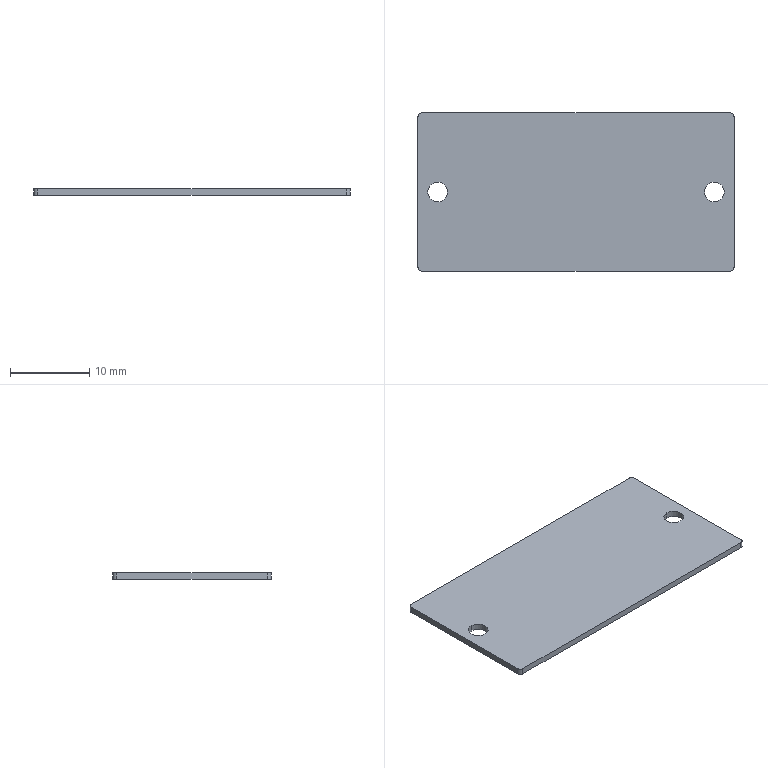Part | STEP file | Nameplate | 1 solid | 14 faces | box 40 x 20 x 0.8 mm | volume 631.974 mm3 | cylinder 8 | plane 6 | commonest cylinder face diameters 1 x4 2.5 x4
STEP:
#1=CARTESIAN_POINT('',(0.,0.,0.));
#2=DIRECTION('',(0.,0.,1.));
#3=DIRECTION('',(1.,0.,0.));
#4=AXIS2_PLACEMENT_3D('',#1,#2,#3);
#5=CARTESIAN_POINT('',(37.5,11.25,0.8));
#6=VERTEX_POINT('',#5);
#7=CARTESIAN_POINT('',(37.5,11.25,0.));
#8=VERTEX_POINT('',#7);
#9=CARTESIAN_POINT('',(37.5,11.25,0.8));
#10=DIRECTION('',(0.,0.,-1.));
#11=VECTOR('',#10,1.);
#12=LINE('',#9,#11);
#13=CARTESIAN_POINT('',(37.5,10.,0.8));
#14=DIRECTION('',(0.,0.,-1.));
#15=DIRECTION('',(0.,1.,0.));
#16=AXIS2_PLACEMENT_3D('',#13,#14,#15);
#17=CYLINDRICAL_SURFACE('',#16,1.25);
#18=CARTESIAN_POINT('',(6.283,0.));
#19=DIRECTION('',(0.,1.));
#20=VECTOR('',#19,1.);
#21=LINE('',#18,#20);
#22=(GEOMETRIC_REPRESENTATION_CONTEXT(2)PARAMETRIC_REPRESENTATION_CONTEXT()REPRESENTATION_CONTEXT('',''));
#23=DEFINITIONAL_REPRESENTATION('',(#21),#22);
#24=PCURVE('',#17,#23);
#25=CARTESIAN_POINT('',(37.5,10.,0.8));
#26=DIRECTION('',(0.,0.,-1.));
#27=DIRECTION('',(0.,1.,0.));
#28=AXIS2_PLACEMENT_3D('',#25,#26,#27);
#29=CYLINDRICAL_SURFACE('',#28,1.25);
#30=CARTESIAN_POINT('',(0.,0.));
#31=DIRECTION('',(0.,1.));
#32=VECTOR('',#31,1.);
#33=LINE('',#30,#32);
#34=(GEOMETRIC_REPRESENTATION_CONTEXT(2)PARAMETRIC_REPRESENTATION_CONTEXT()REPRESENTATION_CONTEXT('',''));
#35=DEFINITIONAL_REPRESENTATION('',(#33),#34);
#36=PCURVE('',#29,#35);
#37=SURFACE_CURVE('',#12,(#24,#36),.PCURVE_S1.);
#38=EDGE_CURVE('',#6,#8,#37,.T.);
#39=ORIENTED_EDGE('',*,*,#38,.T.);
#40=CARTESIAN_POINT('',(37.5,8.75,0.));
#41=VERTEX_POINT('',#40);
#42=CARTESIAN_POINT('',(37.5,10.,0.));
#43=DIRECTION('',(0.,0.,1.));
#44=DIRECTION('',(0.,-1.,0.));
#45=AXIS2_PLACEMENT_3D('',#42,#43,#44);
#46=CIRCLE('',#45,1.25);
#47=CARTESIAN_POINT('',(9.425,0.8));
#48=DIRECTION('',(-1.,0.));
#49=VECTOR('',#48,1.);
#50=LINE('',#47,#49);
#51=(GEOMETRIC_REPRESENTATION_CONTEXT(2)PARAMETRIC_REPRESENTATION_CONTEXT()REPRESENTATION_CONTEXT('',''));
#52=DEFINITIONAL_REPRESENTATION('',(#50),#51);
#53=PCURVE('',#17,#52);
#54=CARTESIAN_POINT('',(20.,0.,0.));
#55=DIRECTION('',(0.,0.,-1.));
#56=DIRECTION('',(0.,1.,0.));
#57=AXIS2_PLACEMENT_3D('',#54,#55,#56);
#58=PLANE('',#57);
#59=CARTESIAN_POINT('',(8.75,17.5));
#60=CARTESIAN_POINT('',(8.75,19.665));
#61=CARTESIAN_POINT('',(10.625,18.583));
#62=CARTESIAN_POINT('',(12.5,17.5));
#63=CARTESIAN_POINT('',(10.625,16.417));
#64=CARTESIAN_POINT('',(8.75,15.335));
#65=CARTESIAN_POINT('',(8.75,17.5));
#66=(BOUNDED_CURVE()B_SPLINE_CURVE(2,(#59,#60,#61,#62,#63,#64,#65),.UNSPECIFIED.,.T.,.F.)B_SPLINE_CURVE_WITH_KNOTS((1,2,2,2,2,1),(-2.094,0.,2.094,4.189,6.283,8.378),.UNSPECIFIED.)CURVE()GEOMETRIC_REPRESENTATION_ITEM()RATIONAL_B_SPLINE_CURVE((1.,0.5,1.,0.5,1.,0.5,1.))REPRESENTATION_ITEM(''));
#67=(GEOMETRIC_REPRESENTATION_CONTEXT(2)PARAMETRIC_REPRESENTATION_CONTEXT()REPRESENTATION_CONTEXT('',''));
#68=DEFINITIONAL_REPRESENTATION('',(#66),#67);
#69=PCURVE('',#58,#68);
#70=SURFACE_CURVE('',#46,(#53,#69),.PCURVE_S1.);
#71=EDGE_CURVE('',#8,#41,#70,.T.);
#72=ORIENTED_EDGE('',*,*,#71,.T.);
#73=CARTESIAN_POINT('',(37.5,8.75,0.8));
#74=VERTEX_POINT('',#73);
#75=CARTESIAN_POINT('',(37.5,8.75,0.8));
#76=DIRECTION('',(0.,0.,-1.));
#77=VECTOR('',#76,1.);
#78=LINE('',#75,#77);
#79=CARTESIAN_POINT('',(3.142,0.));
#80=DIRECTION('',(0.,1.));
#81=VECTOR('',#80,1.);
#82=LINE('',#79,#81);
#83=(GEOMETRIC_REPRESENTATION_CONTEXT(2)PARAMETRIC_REPRESENTATION_CONTEXT()REPRESENTATION_CONTEXT('',''));
#84=DEFINITIONAL_REPRESENTATION('',(#82),#83);
#85=PCURVE('',#17,#84);
#86=CARTESIAN_POINT('',(3.142,0.));
#87=DIRECTION('',(0.,1.));
#88=VECTOR('',#87,1.);
#89=LINE('',#86,#88);
#90=(GEOMETRIC_REPRESENTATION_CONTEXT(2)PARAMETRIC_REPRESENTATION_CONTEXT()REPRESENTATION_CONTEXT('',''));
#91=DEFINITIONAL_REPRESENTATION('',(#89),#90);
#92=PCURVE('',#29,#91);
#93=SURFACE_CURVE('',#78,(#85,#92),.PCURVE_S1.);
#94=EDGE_CURVE('',#74,#41,#93,.T.);
#95=ORIENTED_EDGE('',*,*,#94,.F.);
#96=CARTESIAN_POINT('',(37.5,10.,0.8));
#97=DIRECTION('',(0.,0.,-1.));
#98=DIRECTION('',(0.,1.,0.));
#99=AXIS2_PLACEMENT_3D('',#96,#97,#98);
#100=CIRCLE('',#99,1.25);
#101=CARTESIAN_POINT('',(0.,0.));
#102=DIRECTION('',(1.,0.));
#103=VECTOR('',#102,1.);
#104=LINE('',#101,#103);
#105=(GEOMETRIC_REPRESENTATION_CONTEXT(2)PARAMETRIC_REPRESENTATION_CONTEXT()REPRESENTATION_CONTEXT('',''));
#106=DEFINITIONAL_REPRESENTATION('',(#104),#105);
#107=PCURVE('',#17,#106);
#108=CARTESIAN_POINT('',(20.,0.,0.8));
#109=DIRECTION('',(0.,0.,1.));
#110=DIRECTION('',(0.,-1.,0.));
#111=AXIS2_PLACEMENT_3D('',#108,#109,#110);
#112=PLANE('',#111);
#113=CARTESIAN_POINT('',(-11.25,17.5));
#114=CARTESIAN_POINT('',(-11.25,19.665));
#115=CARTESIAN_POINT('',(-9.375,18.583));
#116=CARTESIAN_POINT('',(-7.5,17.5));
#117=CARTESIAN_POINT('',(-9.375,16.417));
#118=CARTESIAN_POINT('',(-11.25,15.335));
#119=CARTESIAN_POINT('',(-11.25,17.5));
#120=(BOUNDED_CURVE()B_SPLINE_CURVE(2,(#113,#114,#115,#116,#117,#118,#119),.UNSPECIFIED.,.T.,.F.)B_SPLINE_CURVE_WITH_KNOTS((1,2,2,2,2,1),(-2.094,0.,2.094,4.189,6.283,8.378),.UNSPECIFIED.)CURVE()GEOMETRIC_REPRESENTATION_ITEM()RATIONAL_B_SPLINE_CURVE((1.,0.5,1.,0.5,1.,0.5,1.))REPRESENTATION_ITEM(''));
#121=(GEOMETRIC_REPRESENTATION_CONTEXT(2)PARAMETRIC_REPRESENTATION_CONTEXT()REPRESENTATION_CONTEXT('',''));
#122=DEFINITIONAL_REPRESENTATION('',(#120),#121);
#123=PCURVE('',#112,#122);
#124=SURFACE_CURVE('',#100,(#107,#123),.PCURVE_S1.);
#125=EDGE_CURVE('',#74,#6,#124,.T.);
#126=ORIENTED_EDGE('',*,*,#125,.T.);
#127=EDGE_LOOP('',(#39,#72,#95,#126));
#128=FACE_BOUND('',#127,.F.);
#129=ADVANCED_FACE('',(#128),#17,.F.);
#130=CARTESIAN_POINT('',(2.5,11.25,0.8));
#131=VERTEX_POINT('',#130);
#132=CARTESIAN_POINT('',(2.5,11.25,0.));
#133=VERTEX_POINT('',#132);
#134=CARTESIAN_POINT('',(2.5,11.25,0.8));
#135=DIRECTION('',(0.,0.,-1.));
#136=VECTOR('',#135,1.);
#137=LINE('',#134,#136);
#138=CARTESIAN_POINT('',(2.5,10.,0.8));
#139=DIRECTION('',(0.,0.,-1.));
#140=DIRECTION('',(0.,1.,0.));
#141=AXIS2_PLACEMENT_3D('',#138,#139,#140);
#142=CYLINDRICAL_SURFACE('',#141,1.25);
#143=CARTESIAN_POINT('',(6.283,0.));
#144=DIRECTION('',(0.,1.));
#145=VECTOR('',#144,1.);
#146=LINE('',#143,#145);
#147=(GEOMETRIC_REPRESENTATION_CONTEXT(2)PARAMETRIC_REPRESENTATION_CONTEXT()REPRESENTATION_CONTEXT('',''));
#148=DEFINITIONAL_REPRESENTATION('',(#146),#147);
#149=PCURVE('',#142,#148);
#150=CARTESIAN_POINT('',(2.5,10.,0.8));
#151=DIRECTION('',(0.,0.,-1.));
#152=DIRECTION('',(0.,1.,0.));
#153=AXIS2_PLACEMENT_3D('',#150,#151,#152);
#154=CYLINDRICAL_SURFACE('',#153,1.25);
#155=CARTESIAN_POINT('',(0.,0.));
#156=DIRECTION('',(0.,1.));
#157=VECTOR('',#156,1.);
#158=LINE('',#155,#157);
#159=(GEOMETRIC_REPRESENTATION_CONTEXT(2)PARAMETRIC_REPRESENTATION_CONTEXT()REPRESENTATION_CONTEXT('',''));
#160=DEFINITIONAL_REPRESENTATION('',(#158),#159);
#161=PCURVE('',#154,#160);
#162=SURFACE_CURVE('',#137,(#149,#161),.PCURVE_S1.);
#163=EDGE_CURVE('',#131,#133,#162,.T.);
#164=ORIENTED_EDGE('',*,*,#163,.T.);
#165=CARTESIAN_POINT('',(2.5,8.75,0.));
#166=VERTEX_POINT('',#165);
#167=CARTESIAN_POINT('',(2.5,10.,0.));
#168=DIRECTION('',(0.,0.,1.));
#169=DIRECTION('',(0.,-1.,0.));
#170=AXIS2_PLACEMENT_3D('',#167,#168,#169);
#171=CIRCLE('',#170,1.25);
#172=CARTESIAN_POINT('',(9.425,0.8));
#173=DIRECTION('',(-1.,0.));
#174=VECTOR('',#173,1.);
#175=LINE('',#172,#174);
#176=(GEOMETRIC_REPRESENTATION_CONTEXT(2)PARAMETRIC_REPRESENTATION_CONTEXT()REPRESENTATION_CONTEXT('',''));
#177=DEFINITIONAL_REPRESENTATION('',(#175),#176);
#178=PCURVE('',#142,#177);
#179=CARTESIAN_POINT('',(8.75,-17.5));
#180=CARTESIAN_POINT('',(8.75,-15.335));
#181=CARTESIAN_POINT('',(10.625,-16.417));
#182=CARTESIAN_POINT('',(12.5,-17.5));
#183=CARTESIAN_POINT('',(10.625,-18.583));
#184=CARTESIAN_POINT('',(8.75,-19.665));
#185=CARTESIAN_POINT('',(8.75,-17.5));
#186=(BOUNDED_CURVE()B_SPLINE_CURVE(2,(#179,#180,#181,#182,#183,#184,#185),.UNSPECIFIED.,.T.,.F.)B_SPLINE_CURVE_WITH_KNOTS((1,2,2,2,2,1),(-2.094,0.,2.094,4.189,6.283,8.378),.UNSPECIFIED.)CURVE()GEOMETRIC_REPRESENTATION_ITEM()RATIONAL_B_SPLINE_CURVE((1.,0.5,1.,0.5,1.,0.5,1.))REPRESENTATION_ITEM(''));
#187=(GEOMETRIC_REPRESENTATION_CONTEXT(2)PARAMETRIC_REPRESENTATION_CONTEXT()REPRESENTATION_CONTEXT('',''));
#188=DEFINITIONAL_REPRESENTATION('',(#186),#187);
#189=PCURVE('',#58,#188);
#190=SURFACE_CURVE('',#171,(#178,#189),.PCURVE_S1.);
#191=EDGE_CURVE('',#133,#166,#190,.T.);
#192=ORIENTED_EDGE('',*,*,#191,.T.);
#193=CARTESIAN_POINT('',(2.5,8.75,0.8));
#194=VERTEX_POINT('',#193);
#195=CARTESIAN_POINT('',(2.5,8.75,0.8));
#196=DIRECTION('',(0.,0.,-1.));
#197=VECTOR('',#196,1.);
#198=LINE('',#195,#197);
#199=CARTESIAN_POINT('',(3.142,0.));
#200=DIRECTION('',(0.,1.));
#201=VECTOR('',#200,1.);
#202=LINE('',#199,#201);
#203=(GEOMETRIC_REPRESENTATION_CONTEXT(2)PARAMETRIC_REPRESENTATION_CONTEXT()REPRESENTATION_CONTEXT('',''));
#204=DEFINITIONAL_REPRESENTATION('',(#202),#203);
#205=PCURVE('',#142,#204);
#206=CARTESIAN_POINT('',(3.142,0.));
#207=DIRECTION('',(0.,1.));
#208=VECTOR('',#207,1.);
#209=LINE('',#206,#208);
#210=(GEOMETRIC_REPRESENTATION_CONTEXT(2)PARAMETRIC_REPRESENTATION_CONTEXT()REPRESENTATION_CONTEXT('',''));
#211=DEFINITIONAL_REPRESENTATION('',(#209),#210);
#212=PCURVE('',#154,#211);
#213=SURFACE_CURVE('',#198,(#205,#212),.PCURVE_S1.);
#214=EDGE_CURVE('',#194,#166,#213,.T.);
#215=ORIENTED_EDGE('',*,*,#214,.F.);
#216=CARTESIAN_POINT('',(2.5,10.,0.8));
#217=DIRECTION('',(0.,0.,-1.));
#218=DIRECTION('',(0.,1.,0.));
#219=AXIS2_PLACEMENT_3D('',#216,#217,#218);
#220=CIRCLE('',#219,1.25);
#221=CARTESIAN_POINT('',(0.,0.));
#222=DIRECTION('',(1.,0.));
#223=VECTOR('',#222,1.);
#224=LINE('',#221,#223);
#225=(GEOMETRIC_REPRESENTATION_CONTEXT(2)PARAMETRIC_REPRESENTATION_CONTEXT()REPRESENTATION_CONTEXT('',''));
#226=DEFINITIONAL_REPRESENTATION('',(#224),#225);
#227=PCURVE('',#142,#226);
#228=CARTESIAN_POINT('',(-11.25,-17.5));
#229=CARTESIAN_POINT('',(-11.25,-15.335));
#230=CARTESIAN_POINT('',(-9.375,-16.417));
#231=CARTESIAN_POINT('',(-7.5,-17.5));
#232=CARTESIAN_POINT('',(-9.375,-18.583));
#233=CARTESIAN_POINT('',(-11.25,-19.665));
#234=CARTESIAN_POINT('',(-11.25,-17.5));
#235=(BOUNDED_CURVE()B_SPLINE_CURVE(2,(#228,#229,#230,#231,#232,#233,#234),.UNSPECIFIED.,.T.,.F.)B_SPLINE_CURVE_WITH_KNOTS((1,2,2,2,2,1),(-2.094,0.,2.094,4.189,6.283,8.378),.UNSPECIFIED.)CURVE()GEOMETRIC_REPRESENTATION_ITEM()RATIONAL_B_SPLINE_CURVE((1.,0.5,1.,0.5,1.,0.5,1.))REPRESENTATION_ITEM(''));
#236=(GEOMETRIC_REPRESENTATION_CONTEXT(2)PARAMETRIC_REPRESENTATION_CONTEXT()REPRESENTATION_CONTEXT('',''));
#237=DEFINITIONAL_REPRESENTATION('',(#235),#236);
#238=PCURVE('',#112,#237);
#239=SURFACE_CURVE('',#220,(#227,#238),.PCURVE_S1.);
#240=EDGE_CURVE('',#194,#131,#239,.T.);
#241=ORIENTED_EDGE('',*,*,#240,.T.);
#242=EDGE_LOOP('',(#164,#192,#215,#241));
#243=FACE_BOUND('',#242,.F.);
#244=ADVANCED_FACE('',(#243),#142,.F.);
#245=CARTESIAN_POINT('',(0.5,20.,0.));
#246=VERTEX_POINT('',#245);
#247=CARTESIAN_POINT('',(39.5,20.,0.));
#248=VERTEX_POINT('',#247);
#249=CARTESIAN_POINT('',(20.,20.,0.));
#250=DIRECTION('',(1.,0.,0.));
#251=VECTOR('',#250,1.);
#252=LINE('',#249,#251);
#253=CARTESIAN_POINT('',(20.,20.,0.4));
#254=DIRECTION('',(0.,1.,0.));
#255=DIRECTION('',(1.,0.,0.));
#256=AXIS2_PLACEMENT_3D('',#253,#254,#255);
#257=PLANE('',#256);
#258=CARTESIAN_POINT('',(0.,0.4));
#259=DIRECTION('',(1.,0.));
#260=VECTOR('',#259,1.);
#261=LINE('',#258,#260);
#262=(GEOMETRIC_REPRESENTATION_CONTEXT(2)PARAMETRIC_REPRESENTATION_CONTEXT()REPRESENTATION_CONTEXT('',''));
#263=DEFINITIONAL_REPRESENTATION('',(#261),#262);
#264=PCURVE('',#257,#263);
#265=CARTESIAN_POINT('',(20.,0.));
#266=DIRECTION('',(0.,1.));
#267=VECTOR('',#266,1.);
#268=LINE('',#265,#267);
#269=(GEOMETRIC_REPRESENTATION_CONTEXT(2)PARAMETRIC_REPRESENTATION_CONTEXT()REPRESENTATION_CONTEXT('',''));
#270=DEFINITIONAL_REPRESENTATION('',(#268),#269);
#271=PCURVE('',#58,#270);
#272=SURFACE_CURVE('',#252,(#264,#271),.PCURVE_S1.);
#273=EDGE_CURVE('',#246,#248,#272,.T.);
#274=ORIENTED_EDGE('',*,*,#273,.F.);
#275=CARTESIAN_POINT('',(0.5,20.,0.8));
#276=VERTEX_POINT('',#275);
#277=CARTESIAN_POINT('',(0.5,20.,0.4));
#278=DIRECTION('',(0.,0.,1.));
#279=VECTOR('',#278,1.);
#280=LINE('',#277,#279);
#281=CARTESIAN_POINT('',(-19.5,0.));
#282=DIRECTION('',(0.,-1.));
#283=VECTOR('',#282,1.);
#284=LINE('',#281,#283);
#285=(GEOMETRIC_REPRESENTATION_CONTEXT(2)PARAMETRIC_REPRESENTATION_CONTEXT()REPRESENTATION_CONTEXT('',''));
#286=DEFINITIONAL_REPRESENTATION('',(#284),#285);
#287=PCURVE('',#257,#286);
#288=CARTESIAN_POINT('',(0.5,19.5,0.4));
#289=DIRECTION('',(0.,0.,-1.));
#290=DIRECTION('',(0.,1.,0.));
#291=AXIS2_PLACEMENT_3D('',#288,#289,#290);
#292=CYLINDRICAL_SURFACE('',#291,0.5);
#293=CARTESIAN_POINT('',(6.283,0.));
#294=DIRECTION('',(0.,-1.));
#295=VECTOR('',#294,1.);
#296=LINE('',#293,#295);
#297=(GEOMETRIC_REPRESENTATION_CONTEXT(2)PARAMETRIC_REPRESENTATION_CONTEXT()REPRESENTATION_CONTEXT('',''));
#298=DEFINITIONAL_REPRESENTATION('',(#296),#297);
#299=PCURVE('',#292,#298);
#300=SURFACE_CURVE('',#280,(#287,#299),.PCURVE_S1.);
#301=EDGE_CURVE('',#246,#276,#300,.T.);
#302=ORIENTED_EDGE('',*,*,#301,.T.);
#303=CARTESIAN_POINT('',(39.5,20.,0.8));
#304=VERTEX_POINT('',#303);
#305=CARTESIAN_POINT('',(20.,20.,0.8));
#306=DIRECTION('',(-1.,0.,0.));
#307=VECTOR('',#306,1.);
#308=LINE('',#305,#307);
#309=CARTESIAN_POINT('',(0.,-0.4));
#310=DIRECTION('',(-1.,0.));
#311=VECTOR('',#310,1.);
#312=LINE('',#309,#311);
#313=(GEOMETRIC_REPRESENTATION_CONTEXT(2)PARAMETRIC_REPRESENTATION_CONTEXT()REPRESENTATION_CONTEXT('',''));
#314=DEFINITIONAL_REPRESENTATION('',(#312),#313);
#315=PCURVE('',#257,#314);
#316=CARTESIAN_POINT('',(-20.,0.));
#317=DIRECTION('',(0.,-1.));
#318=VECTOR('',#317,1.);
#319=LINE('',#316,#318);
#320=(GEOMETRIC_REPRESENTATION_CONTEXT(2)PARAMETRIC_REPRESENTATION_CONTEXT()REPRESENTATION_CONTEXT('',''));
#321=DEFINITIONAL_REPRESENTATION('',(#319),#320);
#322=PCURVE('',#112,#321);
#323=SURFACE_CURVE('',#308,(#315,#322),.PCURVE_S1.);
#324=EDGE_CURVE('',#304,#276,#323,.T.);
#325=ORIENTED_EDGE('',*,*,#324,.F.);
#326=CARTESIAN_POINT('',(39.5,20.,0.4));
#327=DIRECTION('',(0.,0.,-1.));
#328=VECTOR('',#327,1.);
#329=LINE('',#326,#328);
#330=CARTESIAN_POINT('',(19.5,0.));
#331=DIRECTION('',(0.,1.));
#332=VECTOR('',#331,1.);
#333=LINE('',#330,#332);
#334=(GEOMETRIC_REPRESENTATION_CONTEXT(2)PARAMETRIC_REPRESENTATION_CONTEXT()REPRESENTATION_CONTEXT('',''));
#335=DEFINITIONAL_REPRESENTATION('',(#333),#334);
#336=PCURVE('',#257,#335);
#337=CARTESIAN_POINT('',(39.5,19.5,0.4));
#338=DIRECTION('',(0.,0.,1.));
#339=DIRECTION('',(0.,-1.,0.));
#340=AXIS2_PLACEMENT_3D('',#337,#338,#339);
#341=CYLINDRICAL_SURFACE('',#340,0.5);
#342=CARTESIAN_POINT('',(3.142,0.));
#343=DIRECTION('',(0.,-1.));
#344=VECTOR('',#343,1.);
#345=LINE('',#342,#344);
#346=(GEOMETRIC_REPRESENTATION_CONTEXT(2)PARAMETRIC_REPRESENTATION_CONTEXT()REPRESENTATION_CONTEXT('',''));
#347=DEFINITIONAL_REPRESENTATION('',(#345),#346);
#348=PCURVE('',#341,#347);
#349=SURFACE_CURVE('',#329,(#336,#348),.PCURVE_S1.);
#350=EDGE_CURVE('',#304,#248,#349,.T.);
#351=ORIENTED_EDGE('',*,*,#350,.T.);
#352=EDGE_LOOP('',(#274,#302,#325,#351));
#353=FACE_BOUND('',#352,.T.);
#354=ADVANCED_FACE('',(#353),#257,.T.);
#355=CARTESIAN_POINT('',(37.5,10.,0.8));
#356=DIRECTION('',(0.,0.,-1.));
#357=DIRECTION('',(0.,1.,0.));
#358=AXIS2_PLACEMENT_3D('',#355,#356,#357);
#359=CIRCLE('',#358,1.25);
#360=CARTESIAN_POINT('',(-11.25,17.5));
#361=CARTESIAN_POINT('',(-11.25,19.665));
#362=CARTESIAN_POINT('',(-9.375,18.583));
#363=CARTESIAN_POINT('',(-7.5,17.5));
#364=CARTESIAN_POINT('',(-9.375,16.417));
#365=CARTESIAN_POINT('',(-11.25,15.335));
#366=CARTESIAN_POINT('',(-11.25,17.5));
#367=(BOUNDED_CURVE()B_SPLINE_CURVE(2,(#360,#361,#362,#363,#364,#365,#366),.UNSPECIFIED.,.T.,.F.)B_SPLINE_CURVE_WITH_KNOTS((1,2,2,2,2,1),(-2.094,0.,2.094,4.189,6.283,8.378),.UNSPECIFIED.)CURVE()GEOMETRIC_REPRESENTATION_ITEM()RATIONAL_B_SPLINE_CURVE((1.,0.5,1.,0.5,1.,0.5,1.))REPRESENTATION_ITEM(''));
#368=(GEOMETRIC_REPRESENTATION_CONTEXT(2)PARAMETRIC_REPRESENTATION_CONTEXT()REPRESENTATION_CONTEXT('',''));
#369=DEFINITIONAL_REPRESENTATION('',(#367),#368);
#370=PCURVE('',#112,#369);
#371=CARTESIAN_POINT('',(0.,0.));
#372=DIRECTION('',(1.,0.));
#373=VECTOR('',#372,1.);
#374=LINE('',#371,#373);
#375=(GEOMETRIC_REPRESENTATION_CONTEXT(2)PARAMETRIC_REPRESENTATION_CONTEXT()REPRESENTATION_CONTEXT('',''));
#376=DEFINITIONAL_REPRESENTATION('',(#374),#375);
#377=PCURVE('',#29,#376);
#378=SURFACE_CURVE('',#359,(#370,#377),.PCURVE_S1.);
#379=EDGE_CURVE('',#6,#74,#378,.T.);
#380=ORIENTED_EDGE('',*,*,#379,.T.);
#381=ORIENTED_EDGE('',*,*,#125,.T.);
#382=EDGE_LOOP('',(#380,#381));
#383=FACE_BOUND('',#382,.T.);
#384=CARTESIAN_POINT('',(2.5,10.,0.8));
#385=DIRECTION('',(0.,0.,-1.));
#386=DIRECTION('',(0.,1.,0.));
#387=AXIS2_PLACEMENT_3D('',#384,#385,#386);
#388=CIRCLE('',#387,1.25);
#389=CARTESIAN_POINT('',(-11.25,-17.5));
#390=CARTESIAN_POINT('',(-11.25,-15.335));
#391=CARTESIAN_POINT('',(-9.375,-16.417));
#392=CARTESIAN_POINT('',(-7.5,-17.5));
#393=CARTESIAN_POINT('',(-9.375,-18.583));
#394=CARTESIAN_POINT('',(-11.25,-19.665));
#395=CARTESIAN_POINT('',(-11.25,-17.5));
#396=(BOUNDED_CURVE()B_SPLINE_CURVE(2,(#389,#390,#391,#392,#393,#394,#395),.UNSPECIFIED.,.T.,.F.)B_SPLINE_CURVE_WITH_KNOTS((1,2,2,2,2,1),(-2.094,0.,2.094,4.189,6.283,8.378),.UNSPECIFIED.)CURVE()GEOMETRIC_REPRESENTATION_ITEM()RATIONAL_B_SPLINE_CURVE((1.,0.5,1.,0.5,1.,0.5,1.))REPRESENTATION_ITEM(''));
#397=(GEOMETRIC_REPRESENTATION_CONTEXT(2)PARAMETRIC_REPRESENTATION_CONTEXT()REPRESENTATION_CONTEXT('',''));
#398=DEFINITIONAL_REPRESENTATION('',(#396),#397);
#399=PCURVE('',#112,#398);
#400=CARTESIAN_POINT('',(0.,0.));
#401=DIRECTION('',(1.,0.));
#402=VECTOR('',#401,1.);
#403=LINE('',#400,#402);
#404=(GEOMETRIC_REPRESENTATION_CONTEXT(2)PARAMETRIC_REPRESENTATION_CONTEXT()REPRESENTATION_CONTEXT('',''));
#405=DEFINITIONAL_REPRESENTATION('',(#403),#404);
#406=PCURVE('',#154,#405);
#407=SURFACE_CURVE('',#388,(#399,#406),.PCURVE_S1.);
#408=EDGE_CURVE('',#131,#194,#407,.T.);
#409=ORIENTED_EDGE('',*,*,#408,.T.);
#410=ORIENTED_EDGE('',*,*,#240,.T.);
#411=EDGE_LOOP('',(#409,#410));
#412=FACE_BOUND('',#411,.T.);
#413=CARTESIAN_POINT('',(0.,0.5,0.8));
#414=VERTEX_POINT('',#413);
#415=CARTESIAN_POINT('',(0.,19.5,0.8));
#416=VERTEX_POINT('',#415);
#417=CARTESIAN_POINT('',(0.,0.,0.8));
#418=DIRECTION('',(0.,1.,0.));
#419=VECTOR('',#418,1.);
#420=LINE('',#417,#419);
#421=CARTESIAN_POINT('',(0.,-20.));
#422=DIRECTION('',(-1.,0.));
#423=VECTOR('',#422,1.);
#424=LINE('',#421,#423);
#425=(GEOMETRIC_REPRESENTATION_CONTEXT(2)PARAMETRIC_REPRESENTATION_CONTEXT()REPRESENTATION_CONTEXT('',''));
#426=DEFINITIONAL_REPRESENTATION('',(#424),#425);
#427=PCURVE('',#112,#426);
#428=CARTESIAN_POINT('',(0.,0.,0.4));
#429=DIRECTION('',(-1.,0.,0.));
#430=DIRECTION('',(0.,1.,0.));
#431=AXIS2_PLACEMENT_3D('',#428,#429,#430);
#432=PLANE('',#431);
#433=CARTESIAN_POINT('',(0.,-0.4));
#434=DIRECTION('',(1.,0.));
#435=VECTOR('',#434,1.);
#436=LINE('',#433,#435);
#437=(GEOMETRIC_REPRESENTATION_CONTEXT(2)PARAMETRIC_REPRESENTATION_CONTEXT()REPRESENTATION_CONTEXT('',''));
#438=DEFINITIONAL_REPRESENTATION('',(#436),#437);
#439=PCURVE('',#432,#438);
#440=SURFACE_CURVE('',#420,(#427,#439),.PCURVE_S1.);
#441=EDGE_CURVE('',#414,#416,#440,.T.);
#442=ORIENTED_EDGE('',*,*,#441,.F.);
#443=CARTESIAN_POINT('',(0.5,0.,0.8));
#444=VERTEX_POINT('',#443);
#445=CARTESIAN_POINT('',(0.5,0.5,0.8));
#446=DIRECTION('',(0.,0.,1.));
#447=DIRECTION('',(0.,-1.,0.));
#448=AXIS2_PLACEMENT_3D('',#445,#446,#447);
#449=CIRCLE('',#448,0.5);
#450=CARTESIAN_POINT('',(-0.5,-19.5));
#451=DIRECTION('',(1.,0.));
#452=AXIS2_PLACEMENT_2D('',#450,#451);
#453=CIRCLE('',#452,0.5);
#454=(GEOMETRIC_REPRESENTATION_CONTEXT(2)PARAMETRIC_REPRESENTATION_CONTEXT()REPRESENTATION_CONTEXT('',''));
#455=DEFINITIONAL_REPRESENTATION('',(#453),#454);
#456=PCURVE('',#112,#455);
#457=CARTESIAN_POINT('',(0.5,0.5,0.4));
#458=DIRECTION('',(0.,0.,1.));
#459=DIRECTION('',(0.,-1.,0.));
#460=AXIS2_PLACEMENT_3D('',#457,#458,#459);
#461=CYLINDRICAL_SURFACE('',#460,0.5);
#462=CARTESIAN_POINT('',(0.,0.4));
#463=DIRECTION('',(1.,0.));
#464=VECTOR('',#463,1.);
#465=LINE('',#462,#464);
#466=(GEOMETRIC_REPRESENTATION_CONTEXT(2)PARAMETRIC_REPRESENTATION_CONTEXT()REPRESENTATION_CONTEXT('',''));
#467=DEFINITIONAL_REPRESENTATION('',(#465),#466);
#468=PCURVE('',#461,#467);
#469=SURFACE_CURVE('',#449,(#456,#468),.PCURVE_S1.);
#470=EDGE_CURVE('',#414,#444,#469,.T.);
#471=ORIENTED_EDGE('',*,*,#470,.T.);
#472=CARTESIAN_POINT('',(39.5,0.,0.8));
#473=VERTEX_POINT('',#472);
#474=CARTESIAN_POINT('',(20.,0.,0.8));
#475=DIRECTION('',(1.,0.,0.));
#476=VECTOR('',#475,1.);
#477=LINE('',#474,#476);
#478=CARTESIAN_POINT('',(0.,0.));
#479=DIRECTION('',(0.,1.));
#480=VECTOR('',#479,1.);
#481=LINE('',#478,#480);
#482=(GEOMETRIC_REPRESENTATION_CONTEXT(2)PARAMETRIC_REPRESENTATION_CONTEXT()REPRESENTATION_CONTEXT('',''));
#483=DEFINITIONAL_REPRESENTATION('',(#481),#482);
#484=PCURVE('',#112,#483);
#485=CARTESIAN_POINT('',(20.,0.,0.4));
#486=DIRECTION('',(0.,-1.,0.));
#487=DIRECTION('',(-1.,0.,0.));
#488=AXIS2_PLACEMENT_3D('',#485,#486,#487);
#489=PLANE('',#488);
#490=CARTESIAN_POINT('',(0.,-0.4));
#491=DIRECTION('',(-1.,0.));
#492=VECTOR('',#491,1.);
#493=LINE('',#490,#492);
#494=(GEOMETRIC_REPRESENTATION_CONTEXT(2)PARAMETRIC_REPRESENTATION_CONTEXT()REPRESENTATION_CONTEXT('',''));
#495=DEFINITIONAL_REPRESENTATION('',(#493),#494);
#496=PCURVE('',#489,#495);
#497=SURFACE_CURVE('',#477,(#484,#496),.PCURVE_S1.);
#498=EDGE_CURVE('',#444,#473,#497,.T.);
#499=ORIENTED_EDGE('',*,*,#498,.T.);
#500=CARTESIAN_POINT('',(40.,0.5,0.8));
#501=VERTEX_POINT('',#500);
#502=CARTESIAN_POINT('',(39.5,0.5,0.8));
#503=DIRECTION('',(0.,0.,1.));
#504=DIRECTION('',(0.,-1.,0.));
#505=AXIS2_PLACEMENT_3D('',#502,#503,#504);
#506=CIRCLE('',#505,0.5);
#507=CARTESIAN_POINT('',(-0.5,19.5));
#508=DIRECTION('',(1.,0.));
#509=AXIS2_PLACEMENT_2D('',#507,#508);
#510=CIRCLE('',#509,0.5);
#511=(GEOMETRIC_REPRESENTATION_CONTEXT(2)PARAMETRIC_REPRESENTATION_CONTEXT()REPRESENTATION_CONTEXT('',''));
#512=DEFINITIONAL_REPRESENTATION('',(#510),#511);
#513=PCURVE('',#112,#512);
#514=CARTESIAN_POINT('',(39.5,0.5,0.4));
#515=DIRECTION('',(0.,0.,-1.));
#516=DIRECTION('',(0.,1.,0.));
#517=AXIS2_PLACEMENT_3D('',#514,#515,#516);
#518=CYLINDRICAL_SURFACE('',#517,0.5);
#519=CARTESIAN_POINT('',(3.142,-0.4));
#520=DIRECTION('',(-1.,0.));
#521=VECTOR('',#520,1.);
#522=LINE('',#519,#521);
#523=(GEOMETRIC_REPRESENTATION_CONTEXT(2)PARAMETRIC_REPRESENTATION_CONTEXT()REPRESENTATION_CONTEXT('',''));
#524=DEFINITIONAL_REPRESENTATION('',(#522),#523);
#525=PCURVE('',#518,#524);
#526=SURFACE_CURVE('',#506,(#513,#525),.PCURVE_S1.);
#527=EDGE_CURVE('',#473,#501,#526,.T.);
#528=ORIENTED_EDGE('',*,*,#527,.T.);
#529=CARTESIAN_POINT('',(40.,19.5,0.8));
#530=VERTEX_POINT('',#529);
#531=CARTESIAN_POINT('',(40.,0.,0.8));
#532=DIRECTION('',(0.,1.,0.));
#533=VECTOR('',#532,1.);
#534=LINE('',#531,#533);
#535=CARTESIAN_POINT('',(0.,20.));
#536=DIRECTION('',(-1.,0.));
#537=VECTOR('',#536,1.);
#538=LINE('',#535,#537);
#539=(GEOMETRIC_REPRESENTATION_CONTEXT(2)PARAMETRIC_REPRESENTATION_CONTEXT()REPRESENTATION_CONTEXT('',''));
#540=DEFINITIONAL_REPRESENTATION('',(#538),#539);
#541=PCURVE('',#112,#540);
#542=CARTESIAN_POINT('',(40.,0.,0.4));
#543=DIRECTION('',(1.,0.,0.));
#544=DIRECTION('',(0.,-1.,0.));
#545=AXIS2_PLACEMENT_3D('',#542,#543,#544);
#546=PLANE('',#545);
#547=CARTESIAN_POINT('',(0.,-0.4));
#548=DIRECTION('',(-1.,0.));
#549=VECTOR('',#548,1.);
#550=LINE('',#547,#549);
#551=(GEOMETRIC_REPRESENTATION_CONTEXT(2)PARAMETRIC_REPRESENTATION_CONTEXT()REPRESENTATION_CONTEXT('',''));
#552=DEFINITIONAL_REPRESENTATION('',(#550),#551);
#553=PCURVE('',#546,#552);
#554=SURFACE_CURVE('',#534,(#541,#553),.PCURVE_S1.);
#555=EDGE_CURVE('',#501,#530,#554,.T.);
#556=ORIENTED_EDGE('',*,*,#555,.T.);
#557=CARTESIAN_POINT('',(39.5,19.5,0.8));
#558=DIRECTION('',(0.,0.,1.));
#559=DIRECTION('',(0.,-1.,0.));
#560=AXIS2_PLACEMENT_3D('',#557,#558,#559);
#561=CIRCLE('',#560,0.5);
#562=CARTESIAN_POINT('',(-19.5,19.5));
#563=DIRECTION('',(1.,0.));
#564=AXIS2_PLACEMENT_2D('',#562,#563);
#565=CIRCLE('',#564,0.5);
#566=(GEOMETRIC_REPRESENTATION_CONTEXT(2)PARAMETRIC_REPRESENTATION_CONTEXT()REPRESENTATION_CONTEXT('',''));
#567=DEFINITIONAL_REPRESENTATION('',(#565),#566);
#568=PCURVE('',#112,#567);
#569=CARTESIAN_POINT('',(0.,0.4));
#570=DIRECTION('',(1.,0.));
#571=VECTOR('',#570,1.);
#572=LINE('',#569,#571);
#573=(GEOMETRIC_REPRESENTATION_CONTEXT(2)PARAMETRIC_REPRESENTATION_CONTEXT()REPRESENTATION_CONTEXT('',''));
#574=DEFINITIONAL_REPRESENTATION('',(#572),#573);
#575=PCURVE('',#341,#574);
#576=SURFACE_CURVE('',#561,(#568,#575),.PCURVE_S1.);
#577=EDGE_CURVE('',#530,#304,#576,.T.);
#578=ORIENTED_EDGE('',*,*,#577,.T.);
#579=ORIENTED_EDGE('',*,*,#324,.T.);
#580=CARTESIAN_POINT('',(0.5,19.5,0.8));
#581=DIRECTION('',(0.,0.,1.));
#582=DIRECTION('',(0.,-1.,0.));
#583=AXIS2_PLACEMENT_3D('',#580,#581,#582);
#584=CIRCLE('',#583,0.5);
#585=CARTESIAN_POINT('',(-19.5,-19.5));
#586=DIRECTION('',(1.,0.));
#587=AXIS2_PLACEMENT_2D('',#585,#586);
#588=CIRCLE('',#587,0.5);
#589=(GEOMETRIC_REPRESENTATION_CONTEXT(2)PARAMETRIC_REPRESENTATION_CONTEXT()REPRESENTATION_CONTEXT('',''));
#590=DEFINITIONAL_REPRESENTATION('',(#588),#589);
#591=PCURVE('',#112,#590);
#592=CARTESIAN_POINT('',(9.425,-0.4));
#593=DIRECTION('',(-1.,0.));
#594=VECTOR('',#593,1.);
#595=LINE('',#592,#594);
#596=(GEOMETRIC_REPRESENTATION_CONTEXT(2)PARAMETRIC_REPRESENTATION_CONTEXT()REPRESENTATION_CONTEXT('',''));
#597=DEFINITIONAL_REPRESENTATION('',(#595),#596);
#598=PCURVE('',#292,#597);
#599=SURFACE_CURVE('',#584,(#591,#598),.PCURVE_S1.);
#600=EDGE_CURVE('',#276,#416,#599,.T.);
#601=ORIENTED_EDGE('',*,*,#600,.T.);
#602=EDGE_LOOP('',(#442,#471,#499,#528,#556,#578,#579,#601));
#603=FACE_BOUND('',#602,.T.);
#604=ADVANCED_FACE('',(#383,#412,#603),#112,.T.);
#605=CARTESIAN_POINT('',(0.,0.5,0.));
#606=VERTEX_POINT('',#605);
#607=CARTESIAN_POINT('',(0.,19.5,0.));
#608=VERTEX_POINT('',#607);
#609=CARTESIAN_POINT('',(0.,0.,0.));
#610=DIRECTION('',(0.,1.,0.));
#611=VECTOR('',#610,1.);
#612=LINE('',#609,#611);
#613=CARTESIAN_POINT('',(0.,0.4));
#614=DIRECTION('',(1.,0.));
#615=VECTOR('',#614,1.);
#616=LINE('',#613,#615);
#617=(GEOMETRIC_REPRESENTATION_CONTEXT(2)PARAMETRIC_REPRESENTATION_CONTEXT()REPRESENTATION_CONTEXT('',''));
#618=DEFINITIONAL_REPRESENTATION('',(#616),#617);
#619=PCURVE('',#432,#618);
#620=CARTESIAN_POINT('',(0.,-20.));
#621=DIRECTION('',(1.,0.));
#622=VECTOR('',#621,1.);
#623=LINE('',#620,#622);
#624=(GEOMETRIC_REPRESENTATION_CONTEXT(2)PARAMETRIC_REPRESENTATION_CONTEXT()REPRESENTATION_CONTEXT('',''));
#625=DEFINITIONAL_REPRESENTATION('',(#623),#624);
#626=PCURVE('',#58,#625);
#627=SURFACE_CURVE('',#612,(#619,#626),.PCURVE_S1.);
#628=EDGE_CURVE('',#606,#608,#627,.T.);
#629=ORIENTED_EDGE('',*,*,#628,.F.);
#630=CARTESIAN_POINT('',(0.,0.5,0.4));
#631=DIRECTION('',(0.,0.,1.));
#632=VECTOR('',#631,1.);
#633=LINE('',#630,#632);
#634=CARTESIAN_POINT('',(0.5,0.));
#635=DIRECTION('',(0.,-1.));
#636=VECTOR('',#635,1.);
#637=LINE('',#634,#636);
#638=(GEOMETRIC_REPRESENTATION_CONTEXT(2)PARAMETRIC_REPRESENTATION_CONTEXT()REPRESENTATION_CONTEXT('',''));
#639=DEFINITIONAL_REPRESENTATION('',(#637),#638);
#640=PCURVE('',#432,#639);
#641=CARTESIAN_POINT('',(4.712,0.));
#642=DIRECTION('',(0.,1.));
#643=VECTOR('',#642,1.);
#644=LINE('',#641,#643);
#645=(GEOMETRIC_REPRESENTATION_CONTEXT(2)PARAMETRIC_REPRESENTATION_CONTEXT()REPRESENTATION_CONTEXT('',''));
#646=DEFINITIONAL_REPRESENTATION('',(#644),#645);
#647=PCURVE('',#461,#646);
#648=SURFACE_CURVE('',#633,(#640,#647),.PCURVE_S1.);
#649=EDGE_CURVE('',#606,#414,#648,.T.);
#650=ORIENTED_EDGE('',*,*,#649,.T.);
#651=ORIENTED_EDGE('',*,*,#441,.T.);
#652=CARTESIAN_POINT('',(0.,19.5,0.4));
#653=DIRECTION('',(0.,0.,-1.));
#654=VECTOR('',#653,1.);
#655=LINE('',#652,#654);
#656=CARTESIAN_POINT('',(19.5,0.));
#657=DIRECTION('',(0.,1.));
#658=VECTOR('',#657,1.);
#659=LINE('',#656,#658);
#660=(GEOMETRIC_REPRESENTATION_CONTEXT(2)PARAMETRIC_REPRESENTATION_CONTEXT()REPRESENTATION_CONTEXT('',''));
#661=DEFINITIONAL_REPRESENTATION('',(#659),#660);
#662=PCURVE('',#432,#661);
#663=CARTESIAN_POINT('',(4.712,0.));
#664=DIRECTION('',(0.,1.));
#665=VECTOR('',#664,1.);
#666=LINE('',#663,#665);
#667=(GEOMETRIC_REPRESENTATION_CONTEXT(2)PARAMETRIC_REPRESENTATION_CONTEXT()REPRESENTATION_CONTEXT('',''));
#668=DEFINITIONAL_REPRESENTATION('',(#666),#667);
#669=PCURVE('',#292,#668);
#670=SURFACE_CURVE('',#655,(#662,#669),.PCURVE_S1.);
#671=EDGE_CURVE('',#416,#608,#670,.T.);
#672=ORIENTED_EDGE('',*,*,#671,.T.);
#673=EDGE_LOOP('',(#629,#650,#651,#672));
#674=FACE_BOUND('',#673,.T.);
#675=ADVANCED_FACE('',(#674),#432,.T.);
#676=ORIENTED_EDGE('',*,*,#71,.T.);
#677=CARTESIAN_POINT('',(37.5,10.,0.));
#678=DIRECTION('',(0.,0.,1.));
#679=DIRECTION('',(0.,-1.,0.));
#680=AXIS2_PLACEMENT_3D('',#677,#678,#679);
#681=CIRCLE('',#680,1.25);
#682=CARTESIAN_POINT('',(8.75,17.5));
#683=CARTESIAN_POINT('',(8.75,19.665));
#684=CARTESIAN_POINT('',(10.625,18.583));
#685=CARTESIAN_POINT('',(12.5,17.5));
#686=CARTESIAN_POINT('',(10.625,16.417));
#687=CARTESIAN_POINT('',(8.75,15.335));
#688=CARTESIAN_POINT('',(8.75,17.5));
#689=(BOUNDED_CURVE()B_SPLINE_CURVE(2,(#682,#683,#684,#685,#686,#687,#688),.UNSPECIFIED.,.T.,.F.)B_SPLINE_CURVE_WITH_KNOTS((1,2,2,2,2,1),(-2.094,0.,2.094,4.189,6.283,8.378),.UNSPECIFIED.)CURVE()GEOMETRIC_REPRESENTATION_ITEM()RATIONAL_B_SPLINE_CURVE((1.,0.5,1.,0.5,1.,0.5,1.))REPRESENTATION_ITEM(''));
#690=(GEOMETRIC_REPRESENTATION_CONTEXT(2)PARAMETRIC_REPRESENTATION_CONTEXT()REPRESENTATION_CONTEXT('',''));
#691=DEFINITIONAL_REPRESENTATION('',(#689),#690);
#692=PCURVE('',#58,#691);
#693=CARTESIAN_POINT('',(3.142,0.8));
#694=DIRECTION('',(-1.,0.));
#695=VECTOR('',#694,1.);
#696=LINE('',#693,#695);
#697=(GEOMETRIC_REPRESENTATION_CONTEXT(2)PARAMETRIC_REPRESENTATION_CONTEXT()REPRESENTATION_CONTEXT('',''));
#698=DEFINITIONAL_REPRESENTATION('',(#696),#697);
#699=PCURVE('',#29,#698);
#700=SURFACE_CURVE('',#681,(#692,#699),.PCURVE_S1.);
#701=EDGE_CURVE('',#41,#8,#700,.T.);
#702=ORIENTED_EDGE('',*,*,#701,.T.);
#703=EDGE_LOOP('',(#676,#702));
#704=FACE_BOUND('',#703,.T.);
#705=ORIENTED_EDGE('',*,*,#191,.T.);
#706=CARTESIAN_POINT('',(2.5,10.,0.));
#707=DIRECTION('',(0.,0.,1.));
#708=DIRECTION('',(0.,-1.,0.));
#709=AXIS2_PLACEMENT_3D('',#706,#707,#708);
#710=CIRCLE('',#709,1.25);
#711=CARTESIAN_POINT('',(8.75,-17.5));
#712=CARTESIAN_POINT('',(8.75,-15.335));
#713=CARTESIAN_POINT('',(10.625,-16.417));
#714=CARTESIAN_POINT('',(12.5,-17.5));
#715=CARTESIAN_POINT('',(10.625,-18.583));
#716=CARTESIAN_POINT('',(8.75,-19.665));
#717=CARTESIAN_POINT('',(8.75,-17.5));
#718=(BOUNDED_CURVE()B_SPLINE_CURVE(2,(#711,#712,#713,#714,#715,#716,#717),.UNSPECIFIED.,.T.,.F.)B_SPLINE_CURVE_WITH_KNOTS((1,2,2,2,2,1),(-2.094,0.,2.094,4.189,6.283,8.378),.UNSPECIFIED.)CURVE()GEOMETRIC_REPRESENTATION_ITEM()RATIONAL_B_SPLINE_CURVE((1.,0.5,1.,0.5,1.,0.5,1.))REPRESENTATION_ITEM(''));
#719=(GEOMETRIC_REPRESENTATION_CONTEXT(2)PARAMETRIC_REPRESENTATION_CONTEXT()REPRESENTATION_CONTEXT('',''));
#720=DEFINITIONAL_REPRESENTATION('',(#718),#719);
#721=PCURVE('',#58,#720);
#722=CARTESIAN_POINT('',(3.142,0.8));
#723=DIRECTION('',(-1.,0.));
#724=VECTOR('',#723,1.);
#725=LINE('',#722,#724);
#726=(GEOMETRIC_REPRESENTATION_CONTEXT(2)PARAMETRIC_REPRESENTATION_CONTEXT()REPRESENTATION_CONTEXT('',''));
#727=DEFINITIONAL_REPRESENTATION('',(#725),#726);
#728=PCURVE('',#154,#727);
#729=SURFACE_CURVE('',#710,(#721,#728),.PCURVE_S1.);
#730=EDGE_CURVE('',#166,#133,#729,.T.);
#731=ORIENTED_EDGE('',*,*,#730,.T.);
#732=EDGE_LOOP('',(#705,#731));
#733=FACE_BOUND('',#732,.T.);
#734=CARTESIAN_POINT('',(39.5,0.,0.));
#735=VERTEX_POINT('',#734);
#736=CARTESIAN_POINT('',(0.5,0.,0.));
#737=VERTEX_POINT('',#736);
#738=CARTESIAN_POINT('',(20.,0.,0.));
#739=DIRECTION('',(-1.,0.,0.));
#740=VECTOR('',#739,1.);
#741=LINE('',#738,#740);
#742=CARTESIAN_POINT('',(0.,0.));
#743=DIRECTION('',(0.,-1.));
#744=VECTOR('',#743,1.);
#745=LINE('',#742,#744);
#746=(GEOMETRIC_REPRESENTATION_CONTEXT(2)PARAMETRIC_REPRESENTATION_CONTEXT()REPRESENTATION_CONTEXT('',''));
#747=DEFINITIONAL_REPRESENTATION('',(#745),#746);
#748=PCURVE('',#58,#747);
#749=CARTESIAN_POINT('',(0.,0.4));
#750=DIRECTION('',(1.,0.));
#751=VECTOR('',#750,1.);
#752=LINE('',#749,#751);
#753=(GEOMETRIC_REPRESENTATION_CONTEXT(2)PARAMETRIC_REPRESENTATION_CONTEXT()REPRESENTATION_CONTEXT('',''));
#754=DEFINITIONAL_REPRESENTATION('',(#752),#753);
#755=PCURVE('',#489,#754);
#756=SURFACE_CURVE('',#741,(#748,#755),.PCURVE_S1.);
#757=EDGE_CURVE('',#735,#737,#756,.T.);
#758=ORIENTED_EDGE('',*,*,#757,.T.);
#759=CARTESIAN_POINT('',(0.5,0.5,0.));
#760=DIRECTION('',(0.,0.,-1.));
#761=DIRECTION('',(0.,1.,0.));
#762=AXIS2_PLACEMENT_3D('',#759,#760,#761);
#763=CIRCLE('',#762,0.5);
#764=CARTESIAN_POINT('',(0.5,-19.5));
#765=DIRECTION('',(1.,0.));
#766=AXIS2_PLACEMENT_2D('',#764,#765);
#767=CIRCLE('',#766,0.5);
#768=(GEOMETRIC_REPRESENTATION_CONTEXT(2)PARAMETRIC_REPRESENTATION_CONTEXT()REPRESENTATION_CONTEXT('',''));
#769=DEFINITIONAL_REPRESENTATION('',(#767),#768);
#770=PCURVE('',#58,#769);
#771=CARTESIAN_POINT('',(9.425,-0.4));
#772=DIRECTION('',(-1.,0.));
#773=VECTOR('',#772,1.);
#774=LINE('',#771,#773);
#775=(GEOMETRIC_REPRESENTATION_CONTEXT(2)PARAMETRIC_REPRESENTATION_CONTEXT()REPRESENTATION_CONTEXT('',''));
#776=DEFINITIONAL_REPRESENTATION('',(#774),#775);
#777=PCURVE('',#461,#776);
#778=SURFACE_CURVE('',#763,(#770,#777),.PCURVE_S1.);
#779=EDGE_CURVE('',#737,#606,#778,.T.);
#780=ORIENTED_EDGE('',*,*,#779,.T.);
#781=ORIENTED_EDGE('',*,*,#628,.T.);
#782=CARTESIAN_POINT('',(0.5,19.5,0.));
#783=DIRECTION('',(0.,0.,-1.));
#784=DIRECTION('',(0.,1.,0.));
#785=AXIS2_PLACEMENT_3D('',#782,#783,#784);
#786=CIRCLE('',#785,0.5);
#787=CARTESIAN_POINT('',(19.5,-19.5));
#788=DIRECTION('',(1.,0.));
#789=AXIS2_PLACEMENT_2D('',#787,#788);
#790=CIRCLE('',#789,0.5);
#791=(GEOMETRIC_REPRESENTATION_CONTEXT(2)PARAMETRIC_REPRESENTATION_CONTEXT()REPRESENTATION_CONTEXT('',''));
#792=DEFINITIONAL_REPRESENTATION('',(#790),#791);
#793=PCURVE('',#58,#792);
#794=CARTESIAN_POINT('',(0.,0.4));
#795=DIRECTION('',(1.,0.));
#796=VECTOR('',#795,1.);
#797=LINE('',#794,#796);
#798=(GEOMETRIC_REPRESENTATION_CONTEXT(2)PARAMETRIC_REPRESENTATION_CONTEXT()REPRESENTATION_CONTEXT('',''));
#799=DEFINITIONAL_REPRESENTATION('',(#797),#798);
#800=PCURVE('',#292,#799);
#801=SURFACE_CURVE('',#786,(#793,#800),.PCURVE_S1.);
#802=EDGE_CURVE('',#608,#246,#801,.T.);
#803=ORIENTED_EDGE('',*,*,#802,.T.);
#804=ORIENTED_EDGE('',*,*,#273,.T.);
#805=CARTESIAN_POINT('',(40.,19.5,0.));
#806=VERTEX_POINT('',#805);
#807=CARTESIAN_POINT('',(39.5,19.5,0.));
#808=DIRECTION('',(0.,0.,-1.));
#809=DIRECTION('',(0.,1.,0.));
#810=AXIS2_PLACEMENT_3D('',#807,#808,#809);
#811=CIRCLE('',#810,0.5);
#812=CARTESIAN_POINT('',(19.5,19.5));
#813=DIRECTION('',(1.,0.));
#814=AXIS2_PLACEMENT_2D('',#812,#813);
#815=CIRCLE('',#814,0.5);
#816=(GEOMETRIC_REPRESENTATION_CONTEXT(2)PARAMETRIC_REPRESENTATION_CONTEXT()REPRESENTATION_CONTEXT('',''));
#817=DEFINITIONAL_REPRESENTATION('',(#815),#816);
#818=PCURVE('',#58,#817);
#819=CARTESIAN_POINT('',(3.142,-0.4));
#820=DIRECTION('',(-1.,0.));
#821=VECTOR('',#820,1.);
#822=LINE('',#819,#821);
#823=(GEOMETRIC_REPRESENTATION_CONTEXT(2)PARAMETRIC_REPRESENTATION_CONTEXT()REPRESENTATION_CONTEXT('',''));
#824=DEFINITIONAL_REPRESENTATION('',(#822),#823);
#825=PCURVE('',#341,#824);
#826=SURFACE_CURVE('',#811,(#818,#825),.PCURVE_S1.);
#827=EDGE_CURVE('',#248,#806,#826,.T.);
#828=ORIENTED_EDGE('',*,*,#827,.T.);
#829=CARTESIAN_POINT('',(40.,0.5,0.));
#830=VERTEX_POINT('',#829);
#831=CARTESIAN_POINT('',(40.,0.,0.));
#832=DIRECTION('',(0.,1.,0.));
#833=VECTOR('',#832,1.);
#834=LINE('',#831,#833);
#835=CARTESIAN_POINT('',(0.,20.));
#836=DIRECTION('',(1.,0.));
#837=VECTOR('',#836,1.);
#838=LINE('',#835,#837);
#839=(GEOMETRIC_REPRESENTATION_CONTEXT(2)PARAMETRIC_REPRESENTATION_CONTEXT()REPRESENTATION_CONTEXT('',''));
#840=DEFINITIONAL_REPRESENTATION('',(#838),#839);
#841=PCURVE('',#58,#840);
#842=CARTESIAN_POINT('',(0.,0.4));
#843=DIRECTION('',(-1.,0.));
#844=VECTOR('',#843,1.);
#845=LINE('',#842,#844);
#846=(GEOMETRIC_REPRESENTATION_CONTEXT(2)PARAMETRIC_REPRESENTATION_CONTEXT()REPRESENTATION_CONTEXT('',''));
#847=DEFINITIONAL_REPRESENTATION('',(#845),#846);
#848=PCURVE('',#546,#847);
#849=SURFACE_CURVE('',#834,(#841,#848),.PCURVE_S1.);
#850=EDGE_CURVE('',#830,#806,#849,.T.);
#851=ORIENTED_EDGE('',*,*,#850,.F.);
#852=CARTESIAN_POINT('',(39.5,0.5,0.));
#853=DIRECTION('',(0.,0.,-1.));
#854=DIRECTION('',(0.,1.,0.));
#855=AXIS2_PLACEMENT_3D('',#852,#853,#854);
#856=CIRCLE('',#855,0.5);
#857=CARTESIAN_POINT('',(0.5,19.5));
#858=DIRECTION('',(1.,0.));
#859=AXIS2_PLACEMENT_2D('',#857,#858);
#860=CIRCLE('',#859,0.5);
#861=(GEOMETRIC_REPRESENTATION_CONTEXT(2)PARAMETRIC_REPRESENTATION_CONTEXT()REPRESENTATION_CONTEXT('',''));
#862=DEFINITIONAL_REPRESENTATION('',(#860),#861);
#863=PCURVE('',#58,#862);
#864=CARTESIAN_POINT('',(0.,0.4));
#865=DIRECTION('',(1.,0.));
#866=VECTOR('',#865,1.);
#867=LINE('',#864,#866);
#868=(GEOMETRIC_REPRESENTATION_CONTEXT(2)PARAMETRIC_REPRESENTATION_CONTEXT()REPRESENTATION_CONTEXT('',''));
#869=DEFINITIONAL_REPRESENTATION('',(#867),#868);
#870=PCURVE('',#518,#869);
#871=SURFACE_CURVE('',#856,(#863,#870),.PCURVE_S1.);
#872=EDGE_CURVE('',#830,#735,#871,.T.);
#873=ORIENTED_EDGE('',*,*,#872,.T.);
#874=EDGE_LOOP('',(#758,#780,#781,#803,#804,#828,#851,#873));
#875=FACE_BOUND('',#874,.T.);
#876=ADVANCED_FACE('',(#704,#733,#875),#58,.T.);
#877=ORIENTED_EDGE('',*,*,#498,.F.);
#878=CARTESIAN_POINT('',(0.5,0.,0.4));
#879=DIRECTION('',(0.,0.,-1.));
#880=VECTOR('',#879,1.);
#881=LINE('',#878,#880);
#882=CARTESIAN_POINT('',(19.5,0.));
#883=DIRECTION('',(0.,1.));
#884=VECTOR('',#883,1.);
#885=LINE('',#882,#884);
#886=(GEOMETRIC_REPRESENTATION_CONTEXT(2)PARAMETRIC_REPRESENTATION_CONTEXT()REPRESENTATION_CONTEXT('',''));
#887=DEFINITIONAL_REPRESENTATION('',(#885),#886);
#888=PCURVE('',#489,#887);
#889=CARTESIAN_POINT('',(6.283,0.));
#890=DIRECTION('',(0.,-1.));
#891=VECTOR('',#890,1.);
#892=LINE('',#889,#891);
#893=(GEOMETRIC_REPRESENTATION_CONTEXT(2)PARAMETRIC_REPRESENTATION_CONTEXT()REPRESENTATION_CONTEXT('',''));
#894=DEFINITIONAL_REPRESENTATION('',(#892),#893);
#895=PCURVE('',#461,#894);
#896=SURFACE_CURVE('',#881,(#888,#895),.PCURVE_S1.);
#897=EDGE_CURVE('',#444,#737,#896,.T.);
#898=ORIENTED_EDGE('',*,*,#897,.T.);
#899=ORIENTED_EDGE('',*,*,#757,.F.);
#900=CARTESIAN_POINT('',(39.5,0.,0.4));
#901=DIRECTION('',(0.,0.,1.));
#902=VECTOR('',#901,1.);
#903=LINE('',#900,#902);
#904=CARTESIAN_POINT('',(-19.5,0.));
#905=DIRECTION('',(0.,-1.));
#906=VECTOR('',#905,1.);
#907=LINE('',#904,#906);
#908=(GEOMETRIC_REPRESENTATION_CONTEXT(2)PARAMETRIC_REPRESENTATION_CONTEXT()REPRESENTATION_CONTEXT('',''));
#909=DEFINITIONAL_REPRESENTATION('',(#907),#908);
#910=PCURVE('',#489,#909);
#911=CARTESIAN_POINT('',(3.142,0.));
#912=DIRECTION('',(0.,-1.));
#913=VECTOR('',#912,1.);
#914=LINE('',#911,#913);
#915=(GEOMETRIC_REPRESENTATION_CONTEXT(2)PARAMETRIC_REPRESENTATION_CONTEXT()REPRESENTATION_CONTEXT('',''));
#916=DEFINITIONAL_REPRESENTATION('',(#914),#915);
#917=PCURVE('',#518,#916);
#918=SURFACE_CURVE('',#903,(#910,#917),.PCURVE_S1.);
#919=EDGE_CURVE('',#735,#473,#918,.T.);
#920=ORIENTED_EDGE('',*,*,#919,.T.);
#921=EDGE_LOOP('',(#877,#898,#899,#920));
#922=FACE_BOUND('',#921,.T.);
#923=ADVANCED_FACE('',(#922),#489,.T.);
#924=ORIENTED_EDGE('',*,*,#555,.F.);
#925=CARTESIAN_POINT('',(40.,0.5,0.4));
#926=DIRECTION('',(0.,0.,-1.));
#927=VECTOR('',#926,1.);
#928=LINE('',#925,#927);
#929=CARTESIAN_POINT('',(-0.5,0.));
#930=DIRECTION('',(0.,1.));
#931=VECTOR('',#930,1.);
#932=LINE('',#929,#931);
#933=(GEOMETRIC_REPRESENTATION_CONTEXT(2)PARAMETRIC_REPRESENTATION_CONTEXT()REPRESENTATION_CONTEXT('',''));
#934=DEFINITIONAL_REPRESENTATION('',(#932),#933);
#935=PCURVE('',#546,#934);
#936=CARTESIAN_POINT('',(1.571,0.));
#937=DIRECTION('',(0.,1.));
#938=VECTOR('',#937,1.);
#939=LINE('',#936,#938);
#940=(GEOMETRIC_REPRESENTATION_CONTEXT(2)PARAMETRIC_REPRESENTATION_CONTEXT()REPRESENTATION_CONTEXT('',''));
#941=DEFINITIONAL_REPRESENTATION('',(#939),#940);
#942=PCURVE('',#518,#941);
#943=SURFACE_CURVE('',#928,(#935,#942),.PCURVE_S1.);
#944=EDGE_CURVE('',#501,#830,#943,.T.);
#945=ORIENTED_EDGE('',*,*,#944,.T.);
#946=ORIENTED_EDGE('',*,*,#850,.T.);
#947=CARTESIAN_POINT('',(40.,19.5,0.4));
#948=DIRECTION('',(0.,0.,1.));
#949=VECTOR('',#948,1.);
#950=LINE('',#947,#949);
#951=CARTESIAN_POINT('',(-19.5,0.));
#952=DIRECTION('',(0.,-1.));
#953=VECTOR('',#952,1.);
#954=LINE('',#951,#953);
#955=(GEOMETRIC_REPRESENTATION_CONTEXT(2)PARAMETRIC_REPRESENTATION_CONTEXT()REPRESENTATION_CONTEXT('',''));
#956=DEFINITIONAL_REPRESENTATION('',(#954),#955);
#957=PCURVE('',#546,#956);
#958=CARTESIAN_POINT('',(1.571,0.));
#959=DIRECTION('',(0.,1.));
#960=VECTOR('',#959,1.);
#961=LINE('',#958,#960);
#962=(GEOMETRIC_REPRESENTATION_CONTEXT(2)PARAMETRIC_REPRESENTATION_CONTEXT()REPRESENTATION_CONTEXT('',''));
#963=DEFINITIONAL_REPRESENTATION('',(#961),#962);
#964=PCURVE('',#341,#963);
#965=SURFACE_CURVE('',#950,(#957,#964),.PCURVE_S1.);
#966=EDGE_CURVE('',#806,#530,#965,.T.);
#967=ORIENTED_EDGE('',*,*,#966,.T.);
#968=EDGE_LOOP('',(#924,#945,#946,#967));
#969=FACE_BOUND('',#968,.T.);
#970=ADVANCED_FACE('',(#969),#546,.T.);
#971=ORIENTED_EDGE('',*,*,#827,.F.);
#972=ORIENTED_EDGE('',*,*,#350,.F.);
#973=ORIENTED_EDGE('',*,*,#577,.F.);
#974=ORIENTED_EDGE('',*,*,#966,.F.);
#975=EDGE_LOOP('',(#971,#972,#973,#974));
#976=FACE_BOUND('',#975,.T.);
#977=ADVANCED_FACE('',(#976),#341,.T.);
#978=ORIENTED_EDGE('',*,*,#527,.F.);
#979=ORIENTED_EDGE('',*,*,#919,.F.);
#980=ORIENTED_EDGE('',*,*,#872,.F.);
#981=ORIENTED_EDGE('',*,*,#944,.F.);
#982=EDGE_LOOP('',(#978,#979,#980,#981));
#983=FACE_BOUND('',#982,.T.);
#984=ADVANCED_FACE('',(#983),#518,.T.);
#985=ORIENTED_EDGE('',*,*,#600,.F.);
#986=ORIENTED_EDGE('',*,*,#301,.F.);
#987=ORIENTED_EDGE('',*,*,#802,.F.);
#988=ORIENTED_EDGE('',*,*,#671,.F.);
#989=EDGE_LOOP('',(#985,#986,#987,#988));
#990=FACE_BOUND('',#989,.T.);
#991=ADVANCED_FACE('',(#990),#292,.T.);
#992=ORIENTED_EDGE('',*,*,#779,.F.);
#993=ORIENTED_EDGE('',*,*,#897,.F.);
#994=ORIENTED_EDGE('',*,*,#470,.F.);
#995=ORIENTED_EDGE('',*,*,#649,.F.);
#996=EDGE_LOOP('',(#992,#993,#994,#995));
#997=FACE_BOUND('',#996,.T.);
#998=ADVANCED_FACE('',(#997),#461,.T.);
#999=ORIENTED_EDGE('',*,*,#730,.T.);
#1000=ORIENTED_EDGE('',*,*,#163,.F.);
#1001=ORIENTED_EDGE('',*,*,#408,.T.);
#1002=ORIENTED_EDGE('',*,*,#214,.T.);
#1003=EDGE_LOOP('',(#999,#1000,#1001,#1002));
#1004=FACE_BOUND('',#1003,.F.);
#1005=ADVANCED_FACE('',(#1004),#154,.F.);
#1006=ORIENTED_EDGE('',*,*,#701,.T.);
#1007=ORIENTED_EDGE('',*,*,#38,.F.);
#1008=ORIENTED_EDGE('',*,*,#379,.T.);
#1009=ORIENTED_EDGE('',*,*,#94,.T.);
#1010=EDGE_LOOP('',(#1006,#1007,#1008,#1009));
#1011=FACE_BOUND('',#1010,.F.);
#1012=ADVANCED_FACE('',(#1011),#29,.F.);
#1013=CLOSED_SHELL('',(#129,#244,#354,#604,#675,#876,#923,#970,#977,#984,#991,#998,#1005,#1012));
#1014=MANIFOLD_SOLID_BREP('',#1013);
#1015=(LENGTH_UNIT()NAMED_UNIT(*)SI_UNIT(.MILLI.,.METRE.));
#1016=UNCERTAINTY_MEASURE_WITH_UNIT(LENGTH_MEASURE(0.0000001),#1015,'','');
#1017=(NAMED_UNIT(*)PLANE_ANGLE_UNIT()SI_UNIT($,.RADIAN.));
#1018=(NAMED_UNIT(*)SI_UNIT($,.STERADIAN.)SOLID_ANGLE_UNIT());
#1019=(GEOMETRIC_REPRESENTATION_CONTEXT(3)GLOBAL_UNCERTAINTY_ASSIGNED_CONTEXT((#1016))GLOBAL_UNIT_ASSIGNED_CONTEXT((#1015,#1017,#1018))REPRESENTATION_CONTEXT('',''));
#1020=ADVANCED_BREP_SHAPE_REPRESENTATION('',(#4,#1014),#1019);